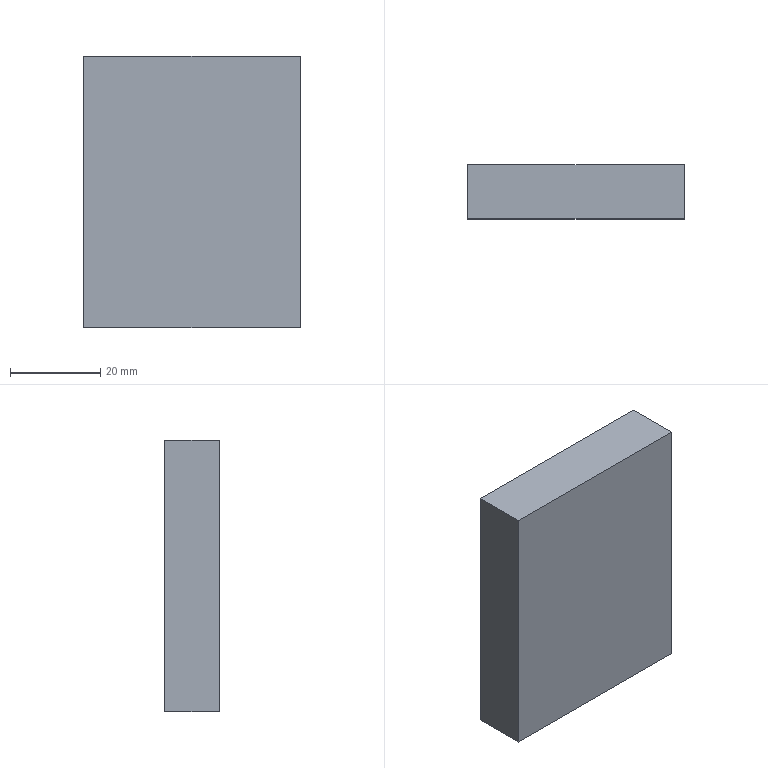Part | SolidWorks | features Extrusion 1 | 1 solid | 6 faces | box 48 x 12 x 60 mm | volume 34560 mm3 | plane 6
STEP:
#1=CARTESIAN_POINT('',(-24.,-6.,30.));
#2=VERTEX_POINT('',#1);
#3=CARTESIAN_POINT('',(24.,-6.,30.));
#4=VERTEX_POINT('',#3);
#5=CARTESIAN_POINT('',(-24.,-6.,30.));
#6=DIRECTION('',(1.,0.,0.));
#7=VECTOR('',#6,1000.);
#8=LINE('',#5,#7);
#9=EDGE_CURVE('',#2,#4,#8,.T.);
#10=ORIENTED_EDGE('',*,*,#9,.T.);
#11=CARTESIAN_POINT('',(24.,6.,30.));
#12=VERTEX_POINT('',#11);
#13=CARTESIAN_POINT('',(24.,6.,30.));
#14=DIRECTION('',(0.,-1.,0.));
#15=VECTOR('',#14,1000.);
#16=LINE('',#13,#15);
#17=EDGE_CURVE('',#12,#4,#16,.T.);
#18=ORIENTED_EDGE('',*,*,#17,.F.);
#19=CARTESIAN_POINT('',(-24.,6.,30.));
#20=VERTEX_POINT('',#19);
#21=CARTESIAN_POINT('',(-24.,6.,30.));
#22=DIRECTION('',(1.,0.,0.));
#23=VECTOR('',#22,1000.);
#24=LINE('',#21,#23);
#25=EDGE_CURVE('',#20,#12,#24,.T.);
#26=ORIENTED_EDGE('',*,*,#25,.F.);
#27=CARTESIAN_POINT('',(-24.,6.,30.));
#28=DIRECTION('',(0.,-1.,0.));
#29=VECTOR('',#28,1000.);
#30=LINE('',#27,#29);
#31=EDGE_CURVE('',#20,#2,#30,.T.);
#32=ORIENTED_EDGE('',*,*,#31,.T.);
#33=EDGE_LOOP('',(#10,#18,#26,#32));
#34=FACE_OUTER_BOUND('',#33,.T.);
#35=CARTESIAN_POINT('',(-24.,6.,30.));
#36=DIRECTION('',(0.,0.,-1.));
#37=DIRECTION('',(-1.,0.,0.));
#38=AXIS2_PLACEMENT_3D('',#35,#36,#37);
#39=PLANE('',#38);
#40=ADVANCED_FACE('',(#34),#39,.F.);
#41=CARTESIAN_POINT('',(24.,-6.,-30.));
#42=VERTEX_POINT('',#41);
#43=CARTESIAN_POINT('',(24.,-6.,30.));
#44=DIRECTION('',(0.,0.,-1.));
#45=VECTOR('',#44,1000.);
#46=LINE('',#43,#45);
#47=EDGE_CURVE('',#4,#42,#46,.T.);
#48=ORIENTED_EDGE('',*,*,#47,.T.);
#49=CARTESIAN_POINT('',(24.,6.,-30.));
#50=VERTEX_POINT('',#49);
#51=CARTESIAN_POINT('',(24.,6.,-30.));
#52=DIRECTION('',(0.,-1.,0.));
#53=VECTOR('',#52,1000.);
#54=LINE('',#51,#53);
#55=EDGE_CURVE('',#50,#42,#54,.T.);
#56=ORIENTED_EDGE('',*,*,#55,.F.);
#57=CARTESIAN_POINT('',(24.,6.,30.));
#58=DIRECTION('',(0.,0.,-1.));
#59=VECTOR('',#58,1000.);
#60=LINE('',#57,#59);
#61=EDGE_CURVE('',#12,#50,#60,.T.);
#62=ORIENTED_EDGE('',*,*,#61,.F.);
#63=ORIENTED_EDGE('',*,*,#17,.T.);
#64=EDGE_LOOP('',(#48,#56,#62,#63));
#65=FACE_OUTER_BOUND('',#64,.T.);
#66=CARTESIAN_POINT('',(24.,6.,30.));
#67=DIRECTION('',(-1.,0.,0.));
#68=DIRECTION('',(0.,0.,1.));
#69=AXIS2_PLACEMENT_3D('',#66,#67,#68);
#70=PLANE('',#69);
#71=ADVANCED_FACE('',(#65),#70,.F.);
#72=CARTESIAN_POINT('',(-24.,-6.,-30.));
#73=VERTEX_POINT('',#72);
#74=CARTESIAN_POINT('',(24.,-6.,-30.));
#75=DIRECTION('',(-1.,0.,0.));
#76=VECTOR('',#75,1000.);
#77=LINE('',#74,#76);
#78=EDGE_CURVE('',#42,#73,#77,.T.);
#79=ORIENTED_EDGE('',*,*,#78,.T.);
#80=CARTESIAN_POINT('',(-24.,6.,-30.));
#81=VERTEX_POINT('',#80);
#82=CARTESIAN_POINT('',(-24.,6.,-30.));
#83=DIRECTION('',(0.,-1.,0.));
#84=VECTOR('',#83,1000.);
#85=LINE('',#82,#84);
#86=EDGE_CURVE('',#81,#73,#85,.T.);
#87=ORIENTED_EDGE('',*,*,#86,.F.);
#88=CARTESIAN_POINT('',(24.,6.,-30.));
#89=DIRECTION('',(-1.,0.,0.));
#90=VECTOR('',#89,1000.);
#91=LINE('',#88,#90);
#92=EDGE_CURVE('',#50,#81,#91,.T.);
#93=ORIENTED_EDGE('',*,*,#92,.F.);
#94=ORIENTED_EDGE('',*,*,#55,.T.);
#95=EDGE_LOOP('',(#79,#87,#93,#94));
#96=FACE_OUTER_BOUND('',#95,.T.);
#97=CARTESIAN_POINT('',(24.,6.,-30.));
#98=DIRECTION('',(0.,0.,1.));
#99=DIRECTION('',(1.,0.,0.));
#100=AXIS2_PLACEMENT_3D('',#97,#98,#99);
#101=PLANE('',#100);
#102=ADVANCED_FACE('',(#96),#101,.F.);
#103=CARTESIAN_POINT('',(-24.,-6.,-30.));
#104=DIRECTION('',(0.,0.,1.));
#105=VECTOR('',#104,1000.);
#106=LINE('',#103,#105);
#107=EDGE_CURVE('',#73,#2,#106,.T.);
#108=ORIENTED_EDGE('',*,*,#107,.T.);
#109=ORIENTED_EDGE('',*,*,#31,.F.);
#110=CARTESIAN_POINT('',(-24.,6.,-30.));
#111=DIRECTION('',(0.,0.,1.));
#112=VECTOR('',#111,1000.);
#113=LINE('',#110,#112);
#114=EDGE_CURVE('',#81,#20,#113,.T.);
#115=ORIENTED_EDGE('',*,*,#114,.F.);
#116=ORIENTED_EDGE('',*,*,#86,.T.);
#117=EDGE_LOOP('',(#108,#109,#115,#116));
#118=FACE_OUTER_BOUND('',#117,.T.);
#119=CARTESIAN_POINT('',(-24.,6.,-30.));
#120=DIRECTION('',(1.,0.,0.));
#121=DIRECTION('',(0.,0.,-1.));
#122=AXIS2_PLACEMENT_3D('',#119,#120,#121);
#123=PLANE('',#122);
#124=ADVANCED_FACE('',(#118),#123,.F.);
#125=ORIENTED_EDGE('',*,*,#25,.T.);
#126=ORIENTED_EDGE('',*,*,#61,.T.);
#127=ORIENTED_EDGE('',*,*,#92,.T.);
#128=ORIENTED_EDGE('',*,*,#114,.T.);
#129=EDGE_LOOP('',(#125,#126,#127,#128));
#130=FACE_OUTER_BOUND('',#129,.T.);
#131=CARTESIAN_POINT('',(24.,6.,30.));
#132=DIRECTION('',(0.,1.,0.));
#133=DIRECTION('',(0.,0.,1.));
#134=AXIS2_PLACEMENT_3D('',#131,#132,#133);
#135=PLANE('',#134);
#136=ADVANCED_FACE('',(#130),#135,.T.);
#137=ORIENTED_EDGE('',*,*,#9,.F.);
#138=ORIENTED_EDGE('',*,*,#107,.F.);
#139=ORIENTED_EDGE('',*,*,#78,.F.);
#140=ORIENTED_EDGE('',*,*,#47,.F.);
#141=EDGE_LOOP('',(#137,#138,#139,#140));
#142=FACE_OUTER_BOUND('',#141,.T.);
#143=CARTESIAN_POINT('',(24.,-6.,30.));
#144=DIRECTION('',(0.,1.,0.));
#145=DIRECTION('',(0.,0.,1.));
#146=AXIS2_PLACEMENT_3D('',#143,#144,#145);
#147=PLANE('',#146);
#148=ADVANCED_FACE('',(#142),#147,.F.);
#149=CLOSED_SHELL('',(#40,#71,#102,#124,#136,#148));
#150=MANIFOLD_SOLID_BREP('',#149);
#151=CARTESIAN_POINT('',(0.,0.,0.));
#152=DIRECTION('',(0.,0.,1.));
#153=DIRECTION('',(1.,0.,0.));
#154=AXIS2_PLACEMENT_3D('',#151,#152,#153);
#155=(LENGTH_UNIT()NAMED_UNIT(*)SI_UNIT(.MILLI.,.METRE.));
#156=UNCERTAINTY_MEASURE_WITH_UNIT(LENGTH_MEASURE(0.00001),#155,'','');
#157=(NAMED_UNIT(*)PLANE_ANGLE_UNIT()SI_UNIT($,.RADIAN.));
#158=(NAMED_UNIT(*)SI_UNIT($,.STERADIAN.)SOLID_ANGLE_UNIT());
#159=(GEOMETRIC_REPRESENTATION_CONTEXT(3)GLOBAL_UNCERTAINTY_ASSIGNED_CONTEXT((#156))GLOBAL_UNIT_ASSIGNED_CONTEXT((#155,#157,#158))REPRESENTATION_CONTEXT('',''));
#160=ADVANCED_BREP_SHAPE_REPRESENTATION('',(#150,#154),#159);